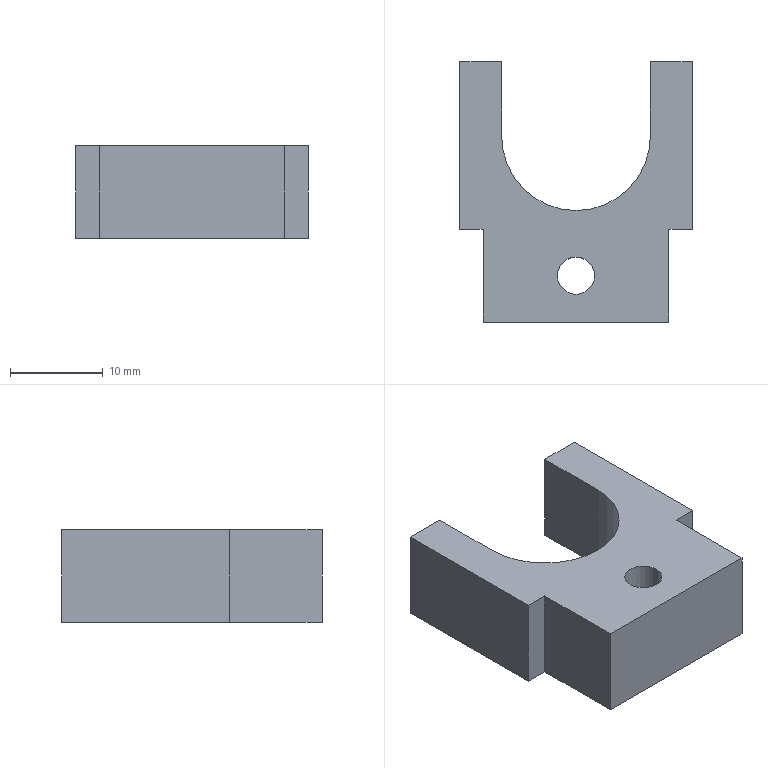Part | SolidWorks | features Extrusion 1 | 1 solid | 16 faces | box 25 x 28 x 10 mm | volume 4089 mm3 | plane 13 | cylinder 3 | commonest cylinder face diameters 4 x2 16 x1
STEP:
#1=CARTESIAN_POINT('',(8.,5.,10.));
#2=VERTEX_POINT('',#1);
#3=CARTESIAN_POINT('',(12.,5.,10.));
#4=VERTEX_POINT('',#3);
#5=CARTESIAN_POINT('',(10.,5.,10.));
#6=DIRECTION('',(0.,0.,1.));
#7=DIRECTION('',(1.,0.,0.));
#8=AXIS2_PLACEMENT_3D('',#5,#6,#7);
#9=CIRCLE('',#8,2.);
#10=EDGE_CURVE('',#2,#4,#9,.T.);
#11=ORIENTED_EDGE('',*,*,#10,.T.);
#12=CARTESIAN_POINT('',(12.,5.,0.));
#13=VERTEX_POINT('',#12);
#14=CARTESIAN_POINT('',(12.,5.,10.));
#15=DIRECTION('',(0.,0.,-1.));
#16=VECTOR('',#15,1000.);
#17=LINE('',#14,#16);
#18=EDGE_CURVE('',#4,#13,#17,.T.);
#19=ORIENTED_EDGE('',*,*,#18,.T.);
#20=CARTESIAN_POINT('',(8.,5.,0.));
#21=VERTEX_POINT('',#20);
#22=CARTESIAN_POINT('',(10.,5.,0.));
#23=DIRECTION('',(0.,0.,1.));
#24=DIRECTION('',(1.,0.,0.));
#25=AXIS2_PLACEMENT_3D('',#22,#23,#24);
#26=CIRCLE('',#25,2.);
#27=EDGE_CURVE('',#21,#13,#26,.T.);
#28=ORIENTED_EDGE('',*,*,#27,.F.);
#29=CARTESIAN_POINT('',(8.,5.,10.));
#30=DIRECTION('',(0.,0.,-1.));
#31=VECTOR('',#30,1000.);
#32=LINE('',#29,#31);
#33=EDGE_CURVE('',#2,#21,#32,.T.);
#34=ORIENTED_EDGE('',*,*,#33,.F.);
#35=EDGE_LOOP('',(#11,#19,#28,#34));
#36=FACE_OUTER_BOUND('',#35,.T.);
#37=CARTESIAN_POINT('',(10.,5.,10.));
#38=DIRECTION('',(0.,0.,-1.));
#39=DIRECTION('',(-1.,0.,0.));
#40=AXIS2_PLACEMENT_3D('',#37,#38,#39);
#41=CYLINDRICAL_SURFACE('',#40,2.);
#42=ADVANCED_FACE('',(#36),#41,.F.);
#43=CARTESIAN_POINT('',(0.,10.,10.));
#44=VERTEX_POINT('',#43);
#45=CARTESIAN_POINT('',(0.,0.,10.));
#46=VERTEX_POINT('',#45);
#47=CARTESIAN_POINT('',(0.,0.,10.));
#48=DIRECTION('',(0.,-1.,0.));
#49=VECTOR('',#48,1000.);
#50=LINE('',#47,#49);
#51=EDGE_CURVE('',#44,#46,#50,.T.);
#52=ORIENTED_EDGE('',*,*,#51,.T.);
#53=CARTESIAN_POINT('',(20.,0.,10.));
#54=VERTEX_POINT('',#53);
#55=CARTESIAN_POINT('',(0.,0.,10.));
#56=DIRECTION('',(1.,0.,0.));
#57=VECTOR('',#56,1000.);
#58=LINE('',#55,#57);
#59=EDGE_CURVE('',#46,#54,#58,.T.);
#60=ORIENTED_EDGE('',*,*,#59,.T.);
#61=CARTESIAN_POINT('',(20.,10.,10.));
#62=VERTEX_POINT('',#61);
#63=CARTESIAN_POINT('',(20.,0.,10.));
#64=DIRECTION('',(0.,1.,0.));
#65=VECTOR('',#64,1000.);
#66=LINE('',#63,#65);
#67=EDGE_CURVE('',#54,#62,#66,.T.);
#68=ORIENTED_EDGE('',*,*,#67,.T.);
#69=CARTESIAN_POINT('',(22.5,10.,10.));
#70=VERTEX_POINT('',#69);
#71=CARTESIAN_POINT('',(20.,10.,10.));
#72=DIRECTION('',(1.,0.,0.));
#73=VECTOR('',#72,1000.);
#74=LINE('',#71,#73);
#75=EDGE_CURVE('',#62,#70,#74,.T.);
#76=ORIENTED_EDGE('',*,*,#75,.T.);
#77=CARTESIAN_POINT('',(22.5,28.,10.));
#78=VERTEX_POINT('',#77);
#79=CARTESIAN_POINT('',(22.5,10.,10.));
#80=DIRECTION('',(0.,1.,0.));
#81=VECTOR('',#80,1000.);
#82=LINE('',#79,#81);
#83=EDGE_CURVE('',#70,#78,#82,.T.);
#84=ORIENTED_EDGE('',*,*,#83,.T.);
#85=CARTESIAN_POINT('',(18.,28.,10.));
#86=VERTEX_POINT('',#85);
#87=CARTESIAN_POINT('',(18.,28.,10.));
#88=DIRECTION('',(-1.,0.,0.));
#89=VECTOR('',#88,1000.);
#90=LINE('',#87,#89);
#91=EDGE_CURVE('',#78,#86,#90,.T.);
#92=ORIENTED_EDGE('',*,*,#91,.T.);
#93=CARTESIAN_POINT('',(18.,20.,10.));
#94=VERTEX_POINT('',#93);
#95=CARTESIAN_POINT('',(18.,20.,10.));
#96=DIRECTION('',(0.,-1.,0.));
#97=VECTOR('',#96,1000.);
#98=LINE('',#95,#97);
#99=EDGE_CURVE('',#86,#94,#98,.T.);
#100=ORIENTED_EDGE('',*,*,#99,.T.);
#101=CARTESIAN_POINT('',(2.,20.,10.));
#102=VERTEX_POINT('',#101);
#103=CARTESIAN_POINT('',(10.,20.,10.));
#104=DIRECTION('',(0.,0.,-1.));
#105=DIRECTION('',(1.,0.,0.));
#106=AXIS2_PLACEMENT_3D('',#103,#104,#105);
#107=CIRCLE('',#106,8.);
#108=EDGE_CURVE('',#94,#102,#107,.T.);
#109=ORIENTED_EDGE('',*,*,#108,.T.);
#110=CARTESIAN_POINT('',(2.,28.,10.));
#111=VERTEX_POINT('',#110);
#112=CARTESIAN_POINT('',(2.,20.,10.));
#113=DIRECTION('',(0.,1.,0.));
#114=VECTOR('',#113,1000.);
#115=LINE('',#112,#114);
#116=EDGE_CURVE('',#102,#111,#115,.T.);
#117=ORIENTED_EDGE('',*,*,#116,.T.);
#118=CARTESIAN_POINT('',(-2.5,28.,10.));
#119=VERTEX_POINT('',#118);
#120=CARTESIAN_POINT('',(2.,28.,10.));
#121=DIRECTION('',(-1.,0.,0.));
#122=VECTOR('',#121,1000.);
#123=LINE('',#120,#122);
#124=EDGE_CURVE('',#111,#119,#123,.T.);
#125=ORIENTED_EDGE('',*,*,#124,.T.);
#126=CARTESIAN_POINT('',(-2.5,10.,10.));
#127=VERTEX_POINT('',#126);
#128=CARTESIAN_POINT('',(-2.5,28.,10.));
#129=DIRECTION('',(0.,-1.,0.));
#130=VECTOR('',#129,1000.);
#131=LINE('',#128,#130);
#132=EDGE_CURVE('',#119,#127,#131,.T.);
#133=ORIENTED_EDGE('',*,*,#132,.T.);
#134=CARTESIAN_POINT('',(0.,10.,10.));
#135=DIRECTION('',(1.,0.,0.));
#136=VECTOR('',#135,1000.);
#137=LINE('',#134,#136);
#138=EDGE_CURVE('',#127,#44,#137,.T.);
#139=ORIENTED_EDGE('',*,*,#138,.T.);
#140=EDGE_LOOP('',(#52,#60,#68,#76,#84,#92,#100,#109,#117,#125,#133,#139));
#141=FACE_OUTER_BOUND('',#140,.T.);
#142=ORIENTED_EDGE('',*,*,#10,.F.);
#143=CARTESIAN_POINT('',(10.,5.,10.));
#144=DIRECTION('',(0.,0.,1.));
#145=DIRECTION('',(1.,0.,0.));
#146=AXIS2_PLACEMENT_3D('',#143,#144,#145);
#147=CIRCLE('',#146,2.);
#148=EDGE_CURVE('',#4,#2,#147,.T.);
#149=ORIENTED_EDGE('',*,*,#148,.F.);
#150=EDGE_LOOP('',(#142,#149));
#151=FACE_BOUND('',#150,.T.);
#152=CARTESIAN_POINT('',(10.,20.,10.));
#153=DIRECTION('',(0.,0.,1.));
#154=DIRECTION('',(1.,0.,0.));
#155=AXIS2_PLACEMENT_3D('',#152,#153,#154);
#156=PLANE('',#155);
#157=ADVANCED_FACE('',(#141,#151),#156,.T.);
#158=CARTESIAN_POINT('',(0.,10.,0.));
#159=VERTEX_POINT('',#158);
#160=CARTESIAN_POINT('',(0.,0.,0.));
#161=VERTEX_POINT('',#160);
#162=CARTESIAN_POINT('',(0.,0.,0.));
#163=DIRECTION('',(0.,-1.,0.));
#164=VECTOR('',#163,1000.);
#165=LINE('',#162,#164);
#166=EDGE_CURVE('',#159,#161,#165,.T.);
#167=ORIENTED_EDGE('',*,*,#166,.F.);
#168=CARTESIAN_POINT('',(-2.5,10.,0.));
#169=VERTEX_POINT('',#168);
#170=CARTESIAN_POINT('',(0.,10.,0.));
#171=DIRECTION('',(1.,0.,0.));
#172=VECTOR('',#171,1000.);
#173=LINE('',#170,#172);
#174=EDGE_CURVE('',#169,#159,#173,.T.);
#175=ORIENTED_EDGE('',*,*,#174,.F.);
#176=CARTESIAN_POINT('',(-2.5,28.,0.));
#177=VERTEX_POINT('',#176);
#178=CARTESIAN_POINT('',(-2.5,10.,0.));
#179=DIRECTION('',(0.,-1.,0.));
#180=VECTOR('',#179,1000.);
#181=LINE('',#178,#180);
#182=EDGE_CURVE('',#177,#169,#181,.T.);
#183=ORIENTED_EDGE('',*,*,#182,.F.);
#184=CARTESIAN_POINT('',(2.,28.,0.));
#185=VERTEX_POINT('',#184);
#186=CARTESIAN_POINT('',(2.,28.,0.));
#187=DIRECTION('',(-1.,0.,0.));
#188=VECTOR('',#187,1000.);
#189=LINE('',#186,#188);
#190=EDGE_CURVE('',#185,#177,#189,.T.);
#191=ORIENTED_EDGE('',*,*,#190,.F.);
#192=CARTESIAN_POINT('',(2.,20.,0.));
#193=VERTEX_POINT('',#192);
#194=CARTESIAN_POINT('',(2.,20.,0.));
#195=DIRECTION('',(0.,1.,0.));
#196=VECTOR('',#195,1000.);
#197=LINE('',#194,#196);
#198=EDGE_CURVE('',#193,#185,#197,.T.);
#199=ORIENTED_EDGE('',*,*,#198,.F.);
#200=CARTESIAN_POINT('',(18.,20.,0.));
#201=VERTEX_POINT('',#200);
#202=CARTESIAN_POINT('',(10.,20.,0.));
#203=DIRECTION('',(0.,0.,-1.));
#204=DIRECTION('',(1.,0.,0.));
#205=AXIS2_PLACEMENT_3D('',#202,#203,#204);
#206=CIRCLE('',#205,8.);
#207=EDGE_CURVE('',#201,#193,#206,.T.);
#208=ORIENTED_EDGE('',*,*,#207,.F.);
#209=CARTESIAN_POINT('',(18.,28.,0.));
#210=VERTEX_POINT('',#209);
#211=CARTESIAN_POINT('',(18.,20.,0.));
#212=DIRECTION('',(0.,-1.,0.));
#213=VECTOR('',#212,1000.);
#214=LINE('',#211,#213);
#215=EDGE_CURVE('',#210,#201,#214,.T.);
#216=ORIENTED_EDGE('',*,*,#215,.F.);
#217=CARTESIAN_POINT('',(22.5,28.,0.));
#218=VERTEX_POINT('',#217);
#219=CARTESIAN_POINT('',(18.,28.,0.));
#220=DIRECTION('',(-1.,0.,0.));
#221=VECTOR('',#220,1000.);
#222=LINE('',#219,#221);
#223=EDGE_CURVE('',#218,#210,#222,.T.);
#224=ORIENTED_EDGE('',*,*,#223,.F.);
#225=CARTESIAN_POINT('',(22.5,10.,0.));
#226=VERTEX_POINT('',#225);
#227=CARTESIAN_POINT('',(22.5,10.,0.));
#228=DIRECTION('',(0.,1.,0.));
#229=VECTOR('',#228,1000.);
#230=LINE('',#227,#229);
#231=EDGE_CURVE('',#226,#218,#230,.T.);
#232=ORIENTED_EDGE('',*,*,#231,.F.);
#233=CARTESIAN_POINT('',(20.,10.,0.));
#234=VERTEX_POINT('',#233);
#235=CARTESIAN_POINT('',(20.,10.,0.));
#236=DIRECTION('',(1.,0.,0.));
#237=VECTOR('',#236,1000.);
#238=LINE('',#235,#237);
#239=EDGE_CURVE('',#234,#226,#238,.T.);
#240=ORIENTED_EDGE('',*,*,#239,.F.);
#241=CARTESIAN_POINT('',(20.,0.,0.));
#242=VERTEX_POINT('',#241);
#243=CARTESIAN_POINT('',(20.,0.,0.));
#244=DIRECTION('',(0.,1.,0.));
#245=VECTOR('',#244,1000.);
#246=LINE('',#243,#245);
#247=EDGE_CURVE('',#242,#234,#246,.T.);
#248=ORIENTED_EDGE('',*,*,#247,.F.);
#249=CARTESIAN_POINT('',(0.,0.,0.));
#250=DIRECTION('',(1.,0.,0.));
#251=VECTOR('',#250,1000.);
#252=LINE('',#249,#251);
#253=EDGE_CURVE('',#161,#242,#252,.T.);
#254=ORIENTED_EDGE('',*,*,#253,.F.);
#255=EDGE_LOOP('',(#167,#175,#183,#191,#199,#208,#216,#224,#232,#240,#248,#254));
#256=FACE_OUTER_BOUND('',#255,.T.);
#257=ORIENTED_EDGE('',*,*,#27,.T.);
#258=CARTESIAN_POINT('',(10.,5.,0.));
#259=DIRECTION('',(0.,0.,1.));
#260=DIRECTION('',(1.,0.,0.));
#261=AXIS2_PLACEMENT_3D('',#258,#259,#260);
#262=CIRCLE('',#261,2.);
#263=EDGE_CURVE('',#13,#21,#262,.T.);
#264=ORIENTED_EDGE('',*,*,#263,.T.);
#265=EDGE_LOOP('',(#257,#264));
#266=FACE_BOUND('',#265,.T.);
#267=CARTESIAN_POINT('',(10.,20.,0.));
#268=DIRECTION('',(0.,0.,1.));
#269=DIRECTION('',(1.,0.,0.));
#270=AXIS2_PLACEMENT_3D('',#267,#268,#269);
#271=PLANE('',#270);
#272=ADVANCED_FACE('',(#256,#266),#271,.F.);
#273=ORIENTED_EDGE('',*,*,#166,.T.);
#274=CARTESIAN_POINT('',(0.,0.,10.));
#275=DIRECTION('',(0.,0.,-1.));
#276=VECTOR('',#275,1000.);
#277=LINE('',#274,#276);
#278=EDGE_CURVE('',#46,#161,#277,.T.);
#279=ORIENTED_EDGE('',*,*,#278,.F.);
#280=ORIENTED_EDGE('',*,*,#51,.F.);
#281=CARTESIAN_POINT('',(0.,10.,10.));
#282=DIRECTION('',(0.,0.,-1.));
#283=VECTOR('',#282,1000.);
#284=LINE('',#281,#283);
#285=EDGE_CURVE('',#44,#159,#284,.T.);
#286=ORIENTED_EDGE('',*,*,#285,.T.);
#287=EDGE_LOOP('',(#273,#279,#280,#286));
#288=FACE_OUTER_BOUND('',#287,.T.);
#289=CARTESIAN_POINT('',(0.,0.,10.));
#290=DIRECTION('',(1.,0.,0.));
#291=DIRECTION('',(0.,1.,0.));
#292=AXIS2_PLACEMENT_3D('',#289,#290,#291);
#293=PLANE('',#292);
#294=ADVANCED_FACE('',(#288),#293,.F.);
#295=ORIENTED_EDGE('',*,*,#253,.T.);
#296=CARTESIAN_POINT('',(20.,0.,10.));
#297=DIRECTION('',(0.,0.,-1.));
#298=VECTOR('',#297,1000.);
#299=LINE('',#296,#298);
#300=EDGE_CURVE('',#54,#242,#299,.T.);
#301=ORIENTED_EDGE('',*,*,#300,.F.);
#302=ORIENTED_EDGE('',*,*,#59,.F.);
#303=ORIENTED_EDGE('',*,*,#278,.T.);
#304=EDGE_LOOP('',(#295,#301,#302,#303));
#305=FACE_OUTER_BOUND('',#304,.T.);
#306=CARTESIAN_POINT('',(0.,0.,10.));
#307=DIRECTION('',(0.,1.,0.));
#308=DIRECTION('',(0.,0.,1.));
#309=AXIS2_PLACEMENT_3D('',#306,#307,#308);
#310=PLANE('',#309);
#311=ADVANCED_FACE('',(#305),#310,.F.);
#312=ORIENTED_EDGE('',*,*,#247,.T.);
#313=CARTESIAN_POINT('',(20.,10.,10.));
#314=DIRECTION('',(0.,0.,-1.));
#315=VECTOR('',#314,1000.);
#316=LINE('',#313,#315);
#317=EDGE_CURVE('',#62,#234,#316,.T.);
#318=ORIENTED_EDGE('',*,*,#317,.F.);
#319=ORIENTED_EDGE('',*,*,#67,.F.);
#320=ORIENTED_EDGE('',*,*,#300,.T.);
#321=EDGE_LOOP('',(#312,#318,#319,#320));
#322=FACE_OUTER_BOUND('',#321,.T.);
#323=CARTESIAN_POINT('',(20.,0.,10.));
#324=DIRECTION('',(-1.,0.,0.));
#325=DIRECTION('',(0.,0.,1.));
#326=AXIS2_PLACEMENT_3D('',#323,#324,#325);
#327=PLANE('',#326);
#328=ADVANCED_FACE('',(#322),#327,.F.);
#329=ORIENTED_EDGE('',*,*,#239,.T.);
#330=CARTESIAN_POINT('',(22.5,10.,10.));
#331=DIRECTION('',(0.,0.,-1.));
#332=VECTOR('',#331,1000.);
#333=LINE('',#330,#332);
#334=EDGE_CURVE('',#70,#226,#333,.T.);
#335=ORIENTED_EDGE('',*,*,#334,.F.);
#336=ORIENTED_EDGE('',*,*,#75,.F.);
#337=ORIENTED_EDGE('',*,*,#317,.T.);
#338=EDGE_LOOP('',(#329,#335,#336,#337));
#339=FACE_OUTER_BOUND('',#338,.T.);
#340=CARTESIAN_POINT('',(20.,10.,10.));
#341=DIRECTION('',(0.,1.,0.));
#342=DIRECTION('',(0.,0.,1.));
#343=AXIS2_PLACEMENT_3D('',#340,#341,#342);
#344=PLANE('',#343);
#345=ADVANCED_FACE('',(#339),#344,.F.);
#346=ORIENTED_EDGE('',*,*,#231,.T.);
#347=CARTESIAN_POINT('',(22.5,28.,10.));
#348=DIRECTION('',(0.,0.,-1.));
#349=VECTOR('',#348,1000.);
#350=LINE('',#347,#349);
#351=EDGE_CURVE('',#78,#218,#350,.T.);
#352=ORIENTED_EDGE('',*,*,#351,.F.);
#353=ORIENTED_EDGE('',*,*,#83,.F.);
#354=ORIENTED_EDGE('',*,*,#334,.T.);
#355=EDGE_LOOP('',(#346,#352,#353,#354));
#356=FACE_OUTER_BOUND('',#355,.T.);
#357=CARTESIAN_POINT('',(22.5,10.,10.));
#358=DIRECTION('',(-1.,0.,0.));
#359=DIRECTION('',(0.,0.,1.));
#360=AXIS2_PLACEMENT_3D('',#357,#358,#359);
#361=PLANE('',#360);
#362=ADVANCED_FACE('',(#356),#361,.F.);
#363=ORIENTED_EDGE('',*,*,#223,.T.);
#364=CARTESIAN_POINT('',(18.,28.,10.));
#365=DIRECTION('',(0.,0.,-1.));
#366=VECTOR('',#365,1000.);
#367=LINE('',#364,#366);
#368=EDGE_CURVE('',#86,#210,#367,.T.);
#369=ORIENTED_EDGE('',*,*,#368,.F.);
#370=ORIENTED_EDGE('',*,*,#91,.F.);
#371=ORIENTED_EDGE('',*,*,#351,.T.);
#372=EDGE_LOOP('',(#363,#369,#370,#371));
#373=FACE_OUTER_BOUND('',#372,.T.);
#374=CARTESIAN_POINT('',(18.,28.,10.));
#375=DIRECTION('',(0.,-1.,0.));
#376=DIRECTION('',(1.,0.,0.));
#377=AXIS2_PLACEMENT_3D('',#374,#375,#376);
#378=PLANE('',#377);
#379=ADVANCED_FACE('',(#373),#378,.F.);
#380=ORIENTED_EDGE('',*,*,#215,.T.);
#381=CARTESIAN_POINT('',(18.,20.,10.));
#382=DIRECTION('',(0.,0.,-1.));
#383=VECTOR('',#382,1000.);
#384=LINE('',#381,#383);
#385=EDGE_CURVE('',#94,#201,#384,.T.);
#386=ORIENTED_EDGE('',*,*,#385,.F.);
#387=ORIENTED_EDGE('',*,*,#99,.F.);
#388=ORIENTED_EDGE('',*,*,#368,.T.);
#389=EDGE_LOOP('',(#380,#386,#387,#388));
#390=FACE_OUTER_BOUND('',#389,.T.);
#391=CARTESIAN_POINT('',(18.,20.,10.));
#392=DIRECTION('',(1.,0.,0.));
#393=DIRECTION('',(0.,0.,-1.));
#394=AXIS2_PLACEMENT_3D('',#391,#392,#393);
#395=PLANE('',#394);
#396=ADVANCED_FACE('',(#390),#395,.F.);
#397=ORIENTED_EDGE('',*,*,#207,.T.);
#398=CARTESIAN_POINT('',(2.,20.,10.));
#399=DIRECTION('',(0.,0.,-1.));
#400=VECTOR('',#399,1000.);
#401=LINE('',#398,#400);
#402=EDGE_CURVE('',#102,#193,#401,.T.);
#403=ORIENTED_EDGE('',*,*,#402,.F.);
#404=ORIENTED_EDGE('',*,*,#108,.F.);
#405=ORIENTED_EDGE('',*,*,#385,.T.);
#406=EDGE_LOOP('',(#397,#403,#404,#405));
#407=FACE_OUTER_BOUND('',#406,.T.);
#408=CARTESIAN_POINT('',(10.,20.,10.));
#409=DIRECTION('',(0.,0.,-1.));
#410=DIRECTION('',(-1.,0.,0.));
#411=AXIS2_PLACEMENT_3D('',#408,#409,#410);
#412=CYLINDRICAL_SURFACE('',#411,8.);
#413=ADVANCED_FACE('',(#407),#412,.F.);
#414=ORIENTED_EDGE('',*,*,#198,.T.);
#415=CARTESIAN_POINT('',(2.,28.,10.));
#416=DIRECTION('',(0.,0.,-1.));
#417=VECTOR('',#416,1000.);
#418=LINE('',#415,#417);
#419=EDGE_CURVE('',#111,#185,#418,.T.);
#420=ORIENTED_EDGE('',*,*,#419,.F.);
#421=ORIENTED_EDGE('',*,*,#116,.F.);
#422=ORIENTED_EDGE('',*,*,#402,.T.);
#423=EDGE_LOOP('',(#414,#420,#421,#422));
#424=FACE_OUTER_BOUND('',#423,.T.);
#425=CARTESIAN_POINT('',(2.,20.,10.));
#426=DIRECTION('',(-1.,0.,0.));
#427=DIRECTION('',(0.,0.,1.));
#428=AXIS2_PLACEMENT_3D('',#425,#426,#427);
#429=PLANE('',#428);
#430=ADVANCED_FACE('',(#424),#429,.F.);
#431=ORIENTED_EDGE('',*,*,#190,.T.);
#432=CARTESIAN_POINT('',(-2.5,28.,10.));
#433=DIRECTION('',(0.,0.,-1.));
#434=VECTOR('',#433,1000.);
#435=LINE('',#432,#434);
#436=EDGE_CURVE('',#119,#177,#435,.T.);
#437=ORIENTED_EDGE('',*,*,#436,.F.);
#438=ORIENTED_EDGE('',*,*,#124,.F.);
#439=ORIENTED_EDGE('',*,*,#419,.T.);
#440=EDGE_LOOP('',(#431,#437,#438,#439));
#441=FACE_OUTER_BOUND('',#440,.T.);
#442=CARTESIAN_POINT('',(2.,28.,10.));
#443=DIRECTION('',(0.,-1.,0.));
#444=DIRECTION('',(0.,0.,-1.));
#445=AXIS2_PLACEMENT_3D('',#442,#443,#444);
#446=PLANE('',#445);
#447=ADVANCED_FACE('',(#441),#446,.F.);
#448=ORIENTED_EDGE('',*,*,#182,.T.);
#449=CARTESIAN_POINT('',(-2.5,10.,10.));
#450=DIRECTION('',(0.,0.,-1.));
#451=VECTOR('',#450,1000.);
#452=LINE('',#449,#451);
#453=EDGE_CURVE('',#127,#169,#452,.T.);
#454=ORIENTED_EDGE('',*,*,#453,.F.);
#455=ORIENTED_EDGE('',*,*,#132,.F.);
#456=ORIENTED_EDGE('',*,*,#436,.T.);
#457=EDGE_LOOP('',(#448,#454,#455,#456));
#458=FACE_OUTER_BOUND('',#457,.T.);
#459=CARTESIAN_POINT('',(-2.5,10.,10.));
#460=DIRECTION('',(1.,0.,0.));
#461=DIRECTION('',(0.,0.,-1.));
#462=AXIS2_PLACEMENT_3D('',#459,#460,#461);
#463=PLANE('',#462);
#464=ADVANCED_FACE('',(#458),#463,.F.);
#465=ORIENTED_EDGE('',*,*,#174,.T.);
#466=ORIENTED_EDGE('',*,*,#285,.F.);
#467=ORIENTED_EDGE('',*,*,#138,.F.);
#468=ORIENTED_EDGE('',*,*,#453,.T.);
#469=EDGE_LOOP('',(#465,#466,#467,#468));
#470=FACE_OUTER_BOUND('',#469,.T.);
#471=CARTESIAN_POINT('',(0.,10.,10.));
#472=DIRECTION('',(0.,1.,0.));
#473=DIRECTION('',(-1.,0.,0.));
#474=AXIS2_PLACEMENT_3D('',#471,#472,#473);
#475=PLANE('',#474);
#476=ADVANCED_FACE('',(#470),#475,.F.);
#477=ORIENTED_EDGE('',*,*,#18,.F.);
#478=ORIENTED_EDGE('',*,*,#148,.T.);
#479=ORIENTED_EDGE('',*,*,#33,.T.);
#480=ORIENTED_EDGE('',*,*,#263,.F.);
#481=EDGE_LOOP('',(#477,#478,#479,#480));
#482=FACE_OUTER_BOUND('',#481,.T.);
#483=CARTESIAN_POINT('',(10.,5.,10.));
#484=DIRECTION('',(0.,0.,-1.));
#485=DIRECTION('',(-1.,0.,0.));
#486=AXIS2_PLACEMENT_3D('',#483,#484,#485);
#487=CYLINDRICAL_SURFACE('',#486,2.);
#488=ADVANCED_FACE('',(#482),#487,.F.);
#489=CLOSED_SHELL('',(#42,#157,#272,#294,#311,#328,#345,#362,#379,#396,#413,#430,#447,#464,#476,#488));
#490=MANIFOLD_SOLID_BREP('',#489);
#491=CARTESIAN_POINT('',(0.,0.,0.));
#492=DIRECTION('',(0.,0.,1.));
#493=DIRECTION('',(1.,0.,0.));
#494=AXIS2_PLACEMENT_3D('',#491,#492,#493);
#495=(LENGTH_UNIT()NAMED_UNIT(*)SI_UNIT(.MILLI.,.METRE.));
#496=UNCERTAINTY_MEASURE_WITH_UNIT(LENGTH_MEASURE(0.00001),#495,'','');
#497=(NAMED_UNIT(*)PLANE_ANGLE_UNIT()SI_UNIT($,.RADIAN.));
#498=(NAMED_UNIT(*)SI_UNIT($,.STERADIAN.)SOLID_ANGLE_UNIT());
#499=(GEOMETRIC_REPRESENTATION_CONTEXT(3)GLOBAL_UNCERTAINTY_ASSIGNED_CONTEXT((#496))GLOBAL_UNIT_ASSIGNED_CONTEXT((#495,#497,#498))REPRESENTATION_CONTEXT('',''));
#500=ADVANCED_BREP_SHAPE_REPRESENTATION('',(#490,#494),#499);